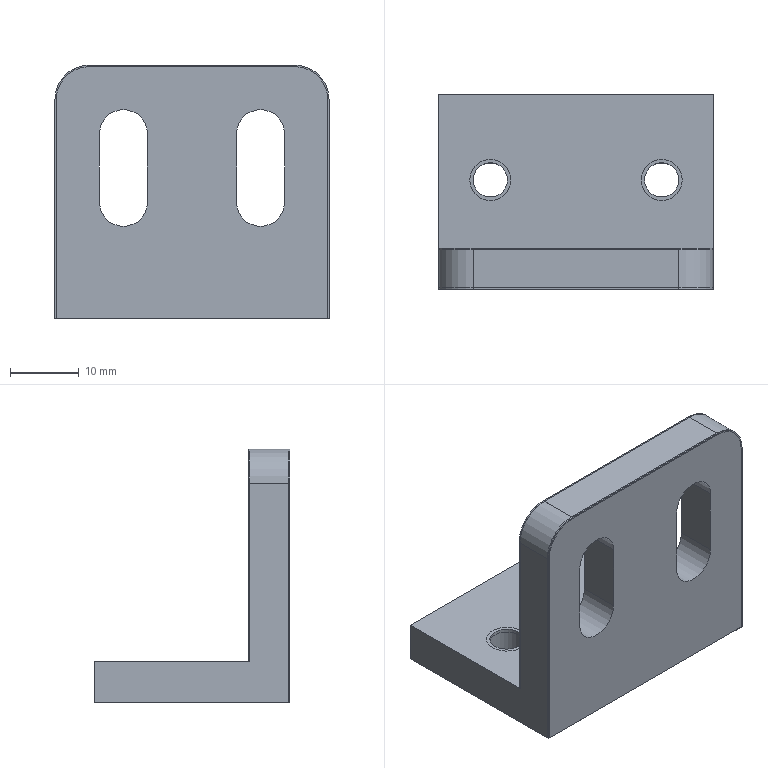NC program | NX | posted with a generic post | part box 40 x 28.5 x 37 mm
Whole program:
N10 G17 G21 G94 G90
(FLOOR_FACING_COPY_2 , TOOL : D63.)
N12 T18 M6
N14 G53
N16 G17 G0 G90 X0. Y61.5 S1500 M3
N18 G43 Z50. H18
N20 Z5.2
N22 G94 G1 Z2.2 F1200.
N24 Y51.5
N26 Y-51.5
N28 Y-61.5
N30 Z5.2
N32 G0 Z50.
N34 Y61.5
N36 Z4.9
N38 G1 Z1.9
N40 Y51.5
N42 Y-51.5
N44 Y-61.5
N46 Z4.9
N48 G0 Z50.
N50 Y61.5
N52 Z4.6
N54 G1 Z1.6
N56 Y51.5
N58 Y-51.5
N60 Y-61.5
N62 Z4.6
N64 G0 Z50.
N66 Y61.5
N68 Z4.3
N70 G1 Z1.3
N72 Y51.5
N74 Y-51.5
N76 Y-61.5
N78 Z4.3
N80 G0 Z50.
N82 Y61.5
N84 Z4.
N86 G1 Z1.
N88 Y51.5
N90 Y-51.5
N92 Y-61.5
N94 Z4.
N96 G0 Z50.
N98 Y61.5
N100 Z3.7
N102 G1 Z0.7
N104 Y51.5
N106 Y-51.5
N108 Y-61.5
N110 Z3.7
N112 G0 Z50.
N114 Y61.5
N116 Z3.4
N118 G1 Z0.4
N120 Y51.5
N122 Y-51.5
N124 Y-61.5
N126 Z3.4
N128 G0 Z50.
N130 Y61.5
N132 Z3.1
N134 G1 Z0.1
N136 Y51.5
N138 Y-51.5
N140 Y-61.5
N142 Z3.1
N144 G0 Z50.
N146 M5
(FLOOR_FACING_COPY_2_COPY , TOOL : D63.J)
N148 T20 M6
N150 G53
N152 G17 G0 G90 X0. Y61.5 S1500 M3
N154 G43 Z50. H20
N156 Z3.
N158 G94 G1 Z0. F400.
N160 Y51.5
N162 Y-51.5
N164 Y-61.5
N166 Z3.
N168 G0 Z50.
N170 M5
(PLANAR_MILL_COPY_COPY_1_1_COPY_COPY , TOOL : 4倒角)
N172 T19 M6
N174 G53
N176 G17 G0 G90 X17.735 Y19.826 S4500 M3
N178 G43 Z50. H19
N180 Z-1.5
N182 G41 G94 G1 X16.75 Y20. F800. D19
N184 X15.75
N186 Y-20.
N188 G2 X14.25 Y-21.5 R1.5
N190 G1 X-14.05
N192 G2 X-15.111 Y-21.061 R1.5
N194 G1 X-15.311 Y-20.861
N196 G2 X-15.75 Y-19.8 R1.5
N198 G1 Y19.8
N200 G2 X-15.311 Y20.861 R1.5
N202 G1 X-15.111 Y21.061
N204 G2 X-14.05 Y21.5 R1.5
N206 G1 X14.25
N208 G2 X15.75 Y20. R1.5
N210 G40
N212 G1 X16.75
N214 G0 Z50.
N216 M5
(DRILLING_COPY , TOOL : D8点钻)
N218 T03 M6
N220 G53
N222 G17 G0 G90 X1.75 Y-12.5 S1500 M3
N224 G43 Z50. H3
N226 G94 G81 G98 Z-3.2 F80. R3.
N228 Y12.5
N230 G80
N232 G0 X1.75 Y12.5 Z50.
N234 M5
(PECK_DRILLING_1 , TOOL : Z5.1)
N236 T06 M6
N238 G53
N240 G17 G0 G90 X1.75 Y-12.5 S1200 M3
N242 G43 Z30. H6
N244 G94 G83 G99 Z-15. F80. Q2. R3.
N246 Y12.5
N248 G80
N250 G0 X1.75 Y12.5 Z30.
N252 M5
N254 M2